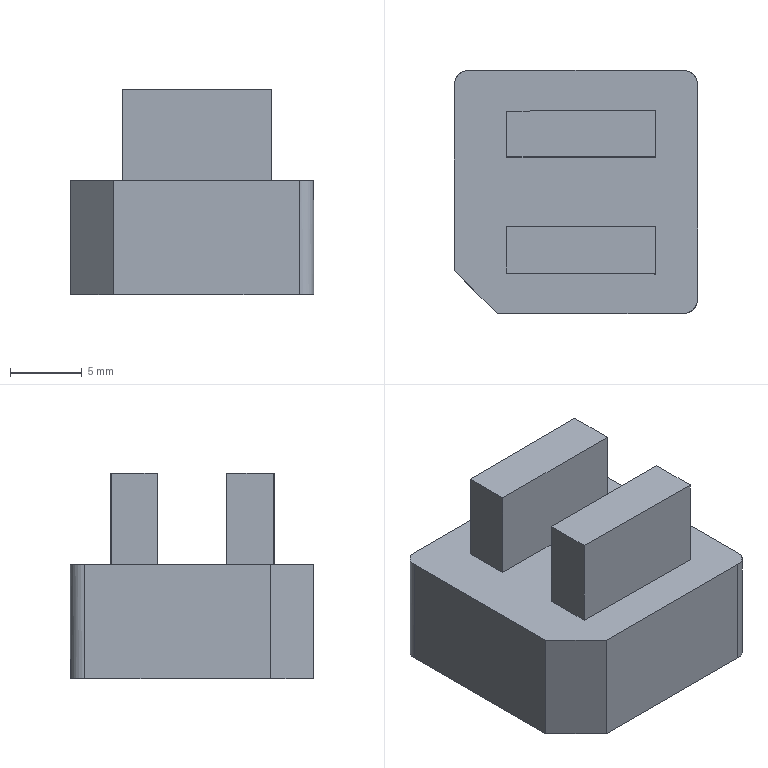NC program | PowerMill | posted with a generic post | part box 17 x 17 x 14.396 mm
Lines 6401 to 7228 of 69084:
N6498 M6
N6499 S8500 M03
N6500 G00 G90 X0.0 Y0.0
N6501 G43 Z11.796 H3
N6502
N6503 G05 P10000 R8
N6504 X16.0978 Y7.7721
N6505 Z0.9258
N6506 G01 Z-0.2742 F360.0
N6507 X10.935 Y6.6897 F600.0
N6508 X-10.201 Y6.6954
N6509 X-10.2583 Y6.3547
N6510 X-10.2871 Y6.09
N6511 X-10.2995 Y5.8905
N6512 X-10.306 Y5.6906
N6513 X-10.3062 Y2.5276
N6514 X-10.3013 Y2.218
N6515 X11.0232 Y2.2123
N6516 X11.002 Y1.899
N6517 X10.9563 Y1.5472
N6518 X10.9195 Y1.3451
N6519 G02 X10.6744 Y0.4925 I-5.5402 J1.1307
N6520 G01 X10.5807 Y0.2614
N6521 X10.4599 Y-0.0004
N6522 X10.5886 Y-0.2788
N6523 X10.7202 Y-0.6192
N6524 X10.788 Y-0.8255
N6525 G02 X11.0078 Y-1.961 I-5.3064 J-1.6164
N6526 G01 X11.0245 Y-2.2651
N6527 X-10.3525 Y-2.2594
N6528 X-10.3562 Y-2.5278
N6529 Y-5.6906
N6530 X-10.3462 Y-6.0157
N6531 X-10.3293 Y-6.2193
N6532 X-10.3062 Y-6.4224
N6533 X-10.2534 Y-6.7368
N6534 X10.9345 Y-6.7424
N6535 G00 Z11.796
N6536 G05 P0
N6537 (---------------)
N6538 ( END TOOLPATH : 精公基准台01-平坦面平行-D10 )
N6539 (---------------)
N6540 ( START TOOLPATH : 精公基准台01-基准面偏置-D10 )
N6541 (---------------)
N6542 G00 X0.0 Y0.0 Z9.7958
N6543 G05 P10000 R8
N6544 X6.0808 Y19.2543
N6545 Z-5.4
N6546 G01 Z-6.6 F360.0
N6547 Y13.9793 F600.0
N6548 X0.2833 Y11.0423
N6549 X5.6668 Y11.0687
N6550 X6.0039 Y11.0503
N6551 X6.2562 Y11.0233
N6552 X6.5169 Y10.982
N6553 X6.8002 Y10.9224
N6554 X7.0836 Y10.8461
N6555 X7.3669 Y10.7534
N6556 X7.6502 Y10.6422
N6557 X7.99 Y10.4837
N6558 X8.2169 Y10.3614
N6559 X8.5003 Y10.1874
N6560 X8.7836 Y9.9881
N6561 X8.876 Y9.917
N6562 X9.1125 Y9.7198
N6563 X9.3503 Y9.4961
N6564 X9.4909 Y9.3503
N6565 X9.718 Y9.0892
N6566 X9.9496 Y8.7836
N6567 X10.1358 Y8.5003
N6568 X10.2977 Y8.2169
N6569 X10.4837 Y7.8312
N6570 X10.5584 Y7.6502
N6571 X10.6604 Y7.3669
N6572 X10.7446 Y7.0836
N6573 X10.8124 Y6.8002
N6574 X10.8644 Y6.5169
N6575 X10.9009 Y6.2335
N6576 X10.922 Y5.9502
N6577 X10.9283 Y5.3835
N6578 X10.9259 Y2.2667
N6579 X10.9098 Y1.9834
N6580 X10.8789 Y1.7001
N6581 X10.832 Y1.4167
N6582 X10.7699 Y1.1334
N6583 X10.6912 Y0.85
N6584 X10.5964 Y0.5689
N6585 X10.5177 Y0.3729
N6586 G03 X10.5175 Y-0.3719 I0.928 J-0.3726
N6587 G01 X10.5969 Y-0.5699
N6588 X10.6915 Y-0.85
N6589 X10.7699 Y-1.1334
N6590 X10.8323 Y-1.4167
N6591 X10.8789 Y-1.7001
N6592 X10.9098 Y-1.9834
N6593 X10.9259 Y-2.2667
N6594 X10.9283 Y-5.3835
N6595 X10.9242 Y-5.9502
N6596 X10.9059 Y-6.2335
N6597 X10.8719 Y-6.5169
N6598 X10.8229 Y-6.8002
N6599 X10.7576 Y-7.0836
N6600 X10.6764 Y-7.3669
N6601 X10.5775 Y-7.6502
N6602 X10.4837 Y-7.881
N6603 X10.324 Y-8.2169
N6604 X10.1659 Y-8.5003
N6605 X9.9842 Y-8.7836
N6606 X9.917 Y-8.8793
N6607 X9.7384 Y-9.1141
N6608 X9.5365 Y-9.3503
N6609 X9.3503 Y-9.5459
N6610 X9.1436 Y-9.7417
N6611 X8.9383 Y-9.917
N6612 X8.7836 Y-10.0379
N6613 X8.5003 Y-10.2372
N6614 X8.2169 Y-10.4109
N6615 X8.0852 Y-10.4837
N6616 X7.8677 Y-10.5939
N6617 X7.6502 Y-10.692
N6618 X7.3669 Y-10.8029
N6619 X7.0836 Y-10.8959
N6620 X6.8002 Y-10.9717
N6621 X6.5169 Y-11.0315
N6622 X6.4076 Y-11.0503
N6623 X5.9502 Y-11.1046
N6624 X5.6668 Y-11.1183
N6625 X-4.8168 Y-11.0653
N6626 X-5.2709 Y-11.0503
N6627 X-5.3835 Y-11.0409
N6628 X-5.6668 Y-11.0065
N6629 X-5.9502 Y-10.9568
N6630 X-6.2335 Y-10.891
N6631 X-6.5169 Y-10.8088
N6632 X-6.8002 Y-10.7091
N6633 X-7.0836 Y-10.5913
N6634 X-7.3085 Y-10.4837
N6635 X-7.6502 Y-10.2947
N6636 X-7.9242 Y-10.1184
N6637 X-8.2169 Y-9.902
N6638 X-8.5003 Y-9.6613
N6639 X-8.6606 Y-9.509
N6640 X-8.8146 Y-9.3503
N6641 X-9.0605 Y-9.0669
N6642 X-9.2745 Y-8.7836
N6643 X-9.3503 Y-8.6729
N6644 X-9.4944 Y-8.4449
N6645 X-9.6234 Y-8.2169
N6646 X-9.764 Y-7.9336
N6647 X-9.8846 Y-7.6502
N6648 X-10.0005 Y-7.3244
N6649 X-10.0714 Y-7.0836
N6650 X-10.1394 Y-6.8002
N6651 X-10.1917 Y-6.5169
N6652 X-10.2284 Y-6.2335
N6653 X-10.2498 Y-5.9502
N6654 X-10.2565 Y-5.3835
N6655 X-10.2538 Y-2.2667
N6656 X-10.2379 Y-1.9834
N6657 X-10.2069 Y-1.7001
N6658 X-10.1602 Y-1.4167
N6659 X-10.098 Y-1.1334
N6660 X-10.0194 Y-0.85
N6661 X-9.917 Y-0.5487
N6662 X-9.8203 Y-0.3092
N6663 G03 X-9.8153 Y0.4265 I-0.9274 J0.3742
N6664 G01 X-9.917 Y0.6887
N6665 X-9.9693 Y0.85
N6666 X-10.048 Y1.1334
N6667 X-10.1101 Y1.4167
N6668 X-10.1566 Y1.7001
N6669 X-10.1879 Y1.9834
N6670 X-10.2039 Y2.2667
N6671 X-10.2064 Y5.3835
N6672 X-10.1973 Y5.9502
N6673 X-10.173 Y6.2335
N6674 X-10.1336 Y6.5169
N6675 X-10.0788 Y6.8002
N6676 X-10.0077 Y7.0836
N6677 X-9.917 Y7.3757
N6678 X-9.8149 Y7.6502
N6679 X-9.6907 Y7.9336
N6680 X-9.5465 Y8.2169
N6681 X-9.3503 Y8.547
N6682 X-9.189 Y8.7836
N6683 X-8.9985 Y9.0319
N6684 X-8.7836 Y9.2803
N6685 X-8.7177 Y9.3503
N6686 X-8.4673 Y9.5962
N6687 X-8.2169 Y9.8127
N6688 X-8.0841 Y9.917
N6689 X-7.8672 Y10.0737
N6690 X-7.6502 Y10.2147
N6691 X-7.4034 Y10.3581
N6692 X-7.0836 Y10.5191
N6693 X-6.8002 Y10.6404
N6694 X-6.5169 Y10.7429
N6695 X-6.2335 Y10.8284
N6696 X-5.9502 Y10.8968
N6697 X-5.6668 Y10.9493
N6698 X-5.3835 Y10.9864
N6699 X-5.1002 Y11.0088
N6700 X-4.8168 Y11.0155
N6701 X0.2833 Y11.0423
N6702 G00 Z9.7958
N6703 G05 P0
N6704 (---------------)
N6705 ( END TOOLPATH : 精公基准台01-基准面偏置-D10 )
N6706 (---------------)
N6707 ( START TOOLPATH : 精公基准台01-外形侧光-D10 )
N6708 (---------------)
N6709 G00 X0.0 Y0.0 Z10.796
N6710 G05 P10000 R8
N6711 X10.9971 Y-1.8364
N6712 Z-5.37
N6713 G01 Z-6.57 F360.0
N6714 G03 X10.5579 Y-2.8971 I1.0608 J-1.0606 F600.0
N6715 G01 X10.5582 Y-5.6597
N6716 G02 X8.5847 Y-9.7236 I-5.0121 J-0.0773
N6717 G02 X5.4763 Y-10.7491 I-3.0386 J3.9866
N6718 G01 X0.2734 Y-10.7218
N6719 X-4.9314 Y-10.6945
N6720 G02 X-9.8863 Y-5.6592 I0.0553 J5.0099
N6721 G01 X-9.8859 Y-2.3708
N6722 G02 X-9.2883 Y-0.0577 I4.9637 J-0.0487
N6723 G03 X-9.2858 Y0.1463 I-0.1936 J0.1043
N6724 G02 X-9.8359 Y2.3732 I4.46 J2.2832
N6725 G01 X-9.8362 Y5.6611
N6726 G02 X-4.9294 Y10.6443 I5.01 J-0.0258
N6727 G01 X5.4771 Y10.6994
N6728 G02 X10.5582 Y5.6592 I0.0702 J-5.0105
N6729 G01 X10.5578 Y2.3708
N6730 G02 X9.9849 Y0.1035 I-4.9764 J0.0514
N6731 G03 X9.9853 Y-0.1044 I0.1941 J-0.1036
N6732 G02 X10.5579 Y-2.3732 I-4.3942 J-2.3155
N6733 G01 Y-2.8971
N6734 G03 X10.9973 Y-3.9577 I1.5 J0.0001
N6735 G01 X10.9171 Y-1.7818
N6736 G03 X10.4779 Y-2.8425 I1.0608 J-1.0605
N6737 G01 X10.4782 Y-5.6592
N6738 G02 X8.5147 Y-9.6763 I-4.932 J-0.0778
N6739 G02 X5.4767 Y-10.6691 I-2.9685 J3.9393
N6740 G01 X0.2738 Y-10.6418
N6741 X-4.929 Y-10.6145
N6742 X-4.9297
N6743 X-4.9305
N6744 G02 X-9.8063 Y-5.6592 I0.0544 J4.9299
N6745 G01 X-9.8059 Y-2.3732
N6746 G02 X-9.2178 Y-0.0957 I4.8836 J-0.0463
N6747 G03 X-9.2145 Y0.1826 I-0.2641 J0.1423
N6748 G02 X-9.7559 Y2.3732 I4.3882 J2.2467
N6749 G01 X-9.7562 Y5.6592
N6750 G02 X-4.929 Y10.5643 I4.9299 J-0.0239
N6751 G01 X5.4767 Y10.6194
N6752 G02 X10.4782 Y5.6592 I0.0706 J-4.9305
N6753 G01 X10.4778 Y2.3732
N6754 G02 X9.9143 Y0.1411 I-4.8961 J0.0489
N6755 G03 X9.9149 Y-0.1424 I0.2647 J-0.1412
N6756 G02 X10.4779 Y-2.3732 I-4.3213 J-2.2769
N6757 G01 Y-2.8425
N6758 G03 X10.9173 Y-3.9031 I1.5 J0.0002
N6759 G00 Z10.796
N6760 G05 P0
N6761 (---------------)
N6762 ( END TOOLPATH : 精公基准台01-外形侧光-D10 )
N6763 (---------------)
N6764 ( START TOOLPATH : 精公基准台01-基准台侧光-D10 )
N6765 (---------------)
N6766 G00 X0.0 Y0.0 Z9.7958
N6767 G05 P10000 R8
N6768 X13.8165 Y-16.5994
N6769 Z-13.3
N6770 G01 Z-14.5 F360.0
N6771 G03 X10.9785 Y-12.4828 I-1.419 J2.0583 F600.0
N6772 G01 X10.7944 Y-12.6097
N6773 X10.7928 Y-12.6108
N6774 X10.7913 Y-12.6118
N6775 X10.6278 Y-12.7137
N6776 X10.6266 Y-12.7144
N6777 X10.6255 Y-12.715
N6778 X10.4729 Y-12.8035
N6779 X10.4714 Y-12.8043
N6780 X10.4698 Y-12.8052
N6781 X10.1537 Y-12.9703
N6782 X10.1516 Y-12.9713
N6783 X10.1495 Y-12.9723
N6784 X9.8333 Y-13.1144
N6785 X9.8312 Y-13.1153
N6786 X9.8291 Y-13.1162
N6787 X9.5129 Y-13.237
N6788 X9.5107 Y-13.2379
N6789 X9.5084 Y-13.2386
N6790 X9.1403 Y-13.3544
N6791 X9.1383 Y-13.3551
N6792 X9.1361 Y-13.3556
N6793 X8.8719 Y-13.4232
N6794 X8.8699 Y-13.4237
N6795 X8.8678 Y-13.4241
N6796 X8.5517 Y-13.4876
N6797 X8.5497 Y-13.488
N6798 X8.5478 Y-13.4883
N6799 X8.2317 Y-13.5357
N6800 X8.2294 Y-13.536
N6801 X8.2271 Y-13.5363
N6802 X7.911 Y-13.5653
N6803 X7.909 Y-13.5655
N6804 X7.9071 Y-13.5656
N6805 X7.5909 Y-13.5792
N6806 X7.5892
N6807 X7.5875
N6808 X-5.3745 Y-13.58
N6809 X-5.3749
N6810 X-5.3754
N6811 X-5.6915 Y-13.5764
N6812 X-5.6939 Y-13.5763
N6813 X-5.6962 Y-13.5762
N6814 X-6.0124 Y-13.5541
N6815 X-6.0149 Y-13.5538
N6816 X-6.0174 Y-13.5535
N6817 X-6.3336 Y-13.5111
N6818 X-6.3361 Y-13.5107
N6819 X-6.3386 Y-13.5103
N6820 X-6.6548 Y-13.447
N6821 X-6.6573 Y-13.4464
N6822 X-6.6598 Y-13.4458
N6823 X-6.976 Y-13.3608
N6824 X-6.9785 Y-13.3601
N6825 X-6.981 Y-13.3593
N6826 X-7.2972 Y-13.2514
N6827 X-7.2997 Y-13.2505
N6828 X-7.3022 Y-13.2495
N6829 X-7.6184 Y-13.1172
N6830 X-7.6203 Y-13.1163
N6831 X-7.6223 Y-13.1154
N6832 X-7.791 Y-13.034
N6833 X-7.7923 Y-13.0334
N6834 X-7.7936 Y-13.0328
N6835 X-7.9409 Y-12.9551
N6836 X-7.9428 Y-12.9541
N6837 X-7.9447 Y-12.953
N6838 X-8.2608 Y-12.7643
N6839 X-8.2624 Y-12.7633
N6840 X-8.2639 Y-12.7623
N6841 X-8.3391 Y-12.7126
N6842 X-8.3404 Y-12.7117
N6843 X-8.3417 Y-12.7108
N6844 X-8.5826 Y-12.5378
N6845 X-8.5843 Y-12.5365
N6846 X-8.5859 Y-12.5352
N6847 X-8.7646 Y-12.3921
N6848 X-8.7659 Y-12.3911
N6849 X-8.7671 Y-12.39
N6850 X-8.9046 Y-12.2703
N6851 X-8.906 Y-12.269
N6852 X-8.9074 Y-12.2678
N6853 X-9.1128 Y-12.0714
N6854 X-9.1135 Y-12.0707
N6855 X-9.1141 Y-12.0701
N6856 X-12.0701 Y-9.1141
N6857 X-12.0707 Y-9.1135
N6858 X-12.0714 Y-9.1128
N6859 X-12.2678 Y-8.9074
N6860 X-12.269 Y-8.906
N6861 X-12.2703 Y-8.9046
N6862 X-12.39 Y-8.7671
N6863 X-12.3911 Y-8.7659
N6864 X-12.3921 Y-8.7646
N6865 X-12.5352 Y-8.5859
N6866 X-12.5365 Y-8.5843
N6867 X-12.5378 Y-8.5826
N6868 X-12.7108 Y-8.3417
N6869 X-12.7117 Y-8.3404
N6870 X-12.7126 Y-8.3391
N6871 X-12.7623 Y-8.2639
N6872 X-12.7633 Y-8.2624
N6873 X-12.7643 Y-8.2608
N6874 X-12.953 Y-7.9447
N6875 X-12.9541 Y-7.9428
N6876 X-12.9551 Y-7.9409
N6877 X-13.0328 Y-7.7936
N6878 X-13.0334 Y-7.7923
N6879 X-13.034 Y-7.791
N6880 X-13.1154 Y-7.6223
N6881 X-13.1163 Y-7.6203
N6882 X-13.1172 Y-7.6184
N6883 X-13.2495 Y-7.3022
N6884 X-13.2505 Y-7.2998
N6885 X-13.2514 Y-7.2973
N6886 X-13.3538 Y-6.9989
N6887 X-13.3546 Y-6.9964
N6888 X-13.3553 Y-6.9939
N6889 X-13.4457 Y-6.66
N6890 X-13.4464 Y-6.6574
N6891 X-13.447 Y-6.6548
N6892 X-13.5103 Y-6.3386
N6893 X-13.5107 Y-6.3361
N6894 X-13.5111 Y-6.3336
N6895 X-13.5535 Y-6.0174
N6896 X-13.5538 Y-6.0149
N6897 X-13.5541 Y-6.0124
N6898 X-13.5762 Y-5.6962
N6899 X-13.5763 Y-5.6939
N6900 X-13.5764 Y-5.6915
N6901 X-13.58 Y-5.3754
N6902 Y-5.3749
N6903 Y-5.3745
N6904 X-13.5792 Y7.5875
N6905 Y7.5891
N6906 Y7.5907
N6907 X-13.5663 Y7.9069
N6908 X-13.5662 Y7.909
N6909 X-13.5661 Y7.9111
N6910 X-13.5363 Y8.2273
N6911 X-13.536 Y8.2294
N6912 X-13.5357 Y8.2315
N6913 X-13.489 Y8.5476
N6914 X-13.4887 Y8.5498
N6915 X-13.4883 Y8.5519
N6916 X-13.424 Y8.868
N6917 X-13.4236 Y8.87
N6918 X-13.4232 Y8.8719
N6919 X-13.3556 Y9.1361
N6920 X-13.3551 Y9.1383
N6921 X-13.3544 Y9.1404
N6922 X-13.2385 Y9.5084
N6923 X-13.2377 Y9.5107
N6924 X-13.2369 Y9.5129
N6925 X-13.1162 Y9.8291
N6926 X-13.1155 Y9.8308
N6927 X-13.1148 Y9.8324
N6928 X-13.0353 Y10.0152
N6929 X-13.0349 Y10.0162
N6930 X-13.0344 Y10.0173
N6931 X-12.9716 Y10.1507
N6932 X-12.9708 Y10.1522
N6933 X-12.9701 Y10.1537
N6934 X-12.8052 Y10.4698
N6935 X-12.8044 Y10.4714
N6936 X-12.8035 Y10.4729
N6937 X-12.715 Y10.6255
N6938 X-12.7144 Y10.6266
N6939 X-12.7137 Y10.6277
N6940 X-12.612 Y10.7912
N6941 X-12.611 Y10.7928
N6942 X-12.6099 Y10.7943
N6943 X-12.3956 Y11.1054
N6944 X-12.394 Y11.1076
N6945 X-12.3924 Y11.1097
N6946 X-12.1383 Y11.4309
N6947 X-12.1372 Y11.4322
N6948 X-12.1362 Y11.4335
N6949 X-12.0741 Y11.5055
N6950 X-12.0732 Y11.5065
N6951 X-12.0722 Y11.5076
N6952 X-11.846 Y11.7518
N6953 X-11.845 Y11.7529
N6954 X-11.8439 Y11.754
N6955 X-11.754 Y11.8439
N6956 X-11.7529 Y11.845
N6957 X-11.7517 Y11.846
N6958 X-11.5074 Y12.0722
N6959 X-11.5062 Y12.0733
N6960 X-11.505 Y12.0744
N6961 X-11.4332 Y12.1357
N6962 X-11.4321 Y12.1367
N6963 X-11.431 Y12.1376
N6964 X-11.1148 Y12.3886
N6965 X-11.1127 Y12.3902
N6966 X-11.1105 Y12.3918
N6967 X-10.7944 Y12.6097
N6968 X-10.7928 Y12.6108
N6969 X-10.7913 Y12.6118
N6970 X-10.6278 Y12.7137
N6971 X-10.6266 Y12.7144
N6972 X-10.6255 Y12.715
N6973 X-10.4729 Y12.8035
N6974 X-10.4714 Y12.8043
N6975 X-10.4698 Y12.8052
N6976 X-10.1537 Y12.9703
N6977 X-10.1516 Y12.9713
N6978 X-10.1495 Y12.9723
N6979 X-9.8333 Y13.1144
N6980 X-9.8312 Y13.1153
N6981 X-9.8291 Y13.1162
N6982 X-9.5129 Y13.237
N6983 X-9.5108 Y13.2378
N6984 X-9.5087 Y13.2385
N6985 X-9.1926 Y13.3396
N6986 X-9.1905 Y13.3402
N6987 X-9.1884 Y13.3408
N6988 X-8.8722 Y13.4231
N6989 X-8.87 Y13.4236
N6990 X-8.8678 Y13.4241
N6991 X-8.5517 Y13.4876
N6992 X-8.5497 Y13.488
N6993 X-8.5478 Y13.4883
N6994 X-8.2317 Y13.5357
N6995 X-8.2294 Y13.536
N6996 X-8.2271 Y13.5363
N6997 X-7.911 Y13.5653
N6998 X-7.909 Y13.5655
N6999 X-7.9071 Y13.5656
N7000 X-7.5909 Y13.5792
N7001 X-7.5892
N7002 X-7.5875
N7003 X0.0
N7004 X7.5875
N7005 X7.5891
N7006 X7.5907
N7007 X7.9069 Y13.5663
N7008 X7.909 Y13.5662
N7009 X7.9111 Y13.5661
N7010 X8.2273 Y13.5363
N7011 X8.2294 Y13.536
N7012 X8.2315 Y13.5357
N7013 X8.5476 Y13.489
N7014 X8.5498 Y13.4887
N7015 X8.5519 Y13.4883
N7016 X8.868 Y13.424
N7017 X8.87 Y13.4236
N7018 X8.8719 Y13.4232
N7019 X9.1361 Y13.3556
N7020 X9.1383 Y13.3551
N7021 X9.1404 Y13.3544
N7022 X9.5084 Y13.2385
N7023 X9.5107 Y13.2377
N7024 X9.5129 Y13.2369
N7025 X9.8291 Y13.1162
N7026 X9.8308 Y13.1155
N7027 X9.8324 Y13.1148
N7028 X10.0152 Y13.0353
N7029 X10.0162 Y13.0349
N7030 X10.0173 Y13.0344
N7031 X10.1507 Y12.9716
N7032 X10.1522 Y12.9708
N7033 X10.1537 Y12.9701
N7034 X10.4698 Y12.8052
N7035 X10.4714 Y12.8044
N7036 X10.4729 Y12.8035
N7037 X10.6255 Y12.715
N7038 X10.6266 Y12.7144
N7039 X10.6277 Y12.7137
N7040 X10.7912 Y12.612
N7041 X10.7928 Y12.611
N7042 X10.7943 Y12.6099
N7043 X11.1054 Y12.3956
N7044 X11.1076 Y12.394
N7045 X11.1097 Y12.3924
N7046 X11.4309 Y12.1383
N7047 X11.4322 Y12.1372
N7048 X11.4335 Y12.1362
N7049 X11.5055 Y12.0741
N7050 X11.5065 Y12.0732
N7051 X11.5076 Y12.0722
N7052 X11.7518 Y11.846
N7053 X11.7529 Y11.845
N7054 X11.754 Y11.8439
N7055 X11.8439 Y11.754
N7056 X11.845 Y11.7529
N7057 X11.846 Y11.7517
N7058 X12.0722 Y11.5074
N7059 X12.0733 Y11.5062
N7060 X12.0744 Y11.505
N7061 X12.1357 Y11.4332
N7062 X12.1367 Y11.4321
N7063 X12.1376 Y11.431
N7064 X12.3886 Y11.1148
N7065 X12.3902 Y11.1127
N7066 X12.3918 Y11.1105
N7067 X12.6097 Y10.7944
N7068 X12.6108 Y10.7928
N7069 X12.6118 Y10.7913
N7070 X12.7137 Y10.6278
N7071 X12.7144 Y10.6266
N7072 X12.715 Y10.6255
N7073 X12.8035 Y10.4729
N7074 X12.8043 Y10.4714
N7075 X12.8052 Y10.4698
N7076 X12.9703 Y10.1537
N7077 X12.9713 Y10.1516
N7078 X12.9723 Y10.1495
N7079 X13.1144 Y9.8333
N7080 X13.1153 Y9.8312
N7081 X13.1162 Y9.8291
N7082 X13.237 Y9.5129
N7083 X13.2378 Y9.5108
N7084 X13.2385 Y9.5087
N7085 X13.3396 Y9.1926
N7086 X13.3402 Y9.1905
N7087 X13.3408 Y9.1884
N7088 X13.4231 Y8.8722
N7089 X13.4236 Y8.87
N7090 X13.4241 Y8.8678
N7091 X13.4876 Y8.5517
N7092 X13.488 Y8.5497
N7093 X13.4883 Y8.5478
N7094 X13.5357 Y8.2317
N7095 X13.536 Y8.2294
N7096 X13.5363 Y8.2271
N7097 X13.5653 Y7.911
N7098 X13.5655 Y7.909
N7099 X13.5656 Y7.9071
N7100 X13.5792 Y7.5909
N7101 Y7.5892
N7102 Y7.5875
N7103 Y-7.5875
N7104 Y-7.5891
N7105 Y-7.5907
N7106 X13.5663 Y-7.9069
N7107 X13.5662 Y-7.909
N7108 X13.5661 Y-7.9111
N7109 X13.5363 Y-8.2273
N7110 X13.536 Y-8.2294
N7111 X13.5357 Y-8.2315
N7112 X13.489 Y-8.5476
N7113 X13.4887 Y-8.5498
N7114 X13.4883 Y-8.5519
N7115 X13.424 Y-8.868
N7116 X13.4236 Y-8.87
N7117 X13.4232 Y-8.8719
N7118 X13.3556 Y-9.1361
N7119 X13.3551 Y-9.1383
N7120 X13.3544 Y-9.1404
N7121 X13.2385 Y-9.5084
N7122 X13.2377 Y-9.5107
N7123 X13.2369 Y-9.5129
N7124 X13.1162 Y-9.8291
N7125 X13.1155 Y-9.8308
N7126 X13.1148 Y-9.8324
N7127 X13.0353 Y-10.0152
N7128 X13.0349 Y-10.0162
N7129 X13.0344 Y-10.0173
N7130 X12.9716 Y-10.1507
N7131 X12.9708 Y-10.1522
N7132 X12.9701 Y-10.1537
N7133 X12.8052 Y-10.4698
N7134 X12.8044 Y-10.4714
N7135 X12.8035 Y-10.4729
N7136 X12.715 Y-10.6255
N7137 X12.7144 Y-10.6266
N7138 X12.7137 Y-10.6277
N7139 X12.612 Y-10.7912
N7140 X12.611 Y-10.7928
N7141 X12.6099 Y-10.7943
N7142 X12.3956 Y-11.1054
N7143 X12.394 Y-11.1076
N7144 X12.3924 Y-11.1097
N7145 X12.1383 Y-11.4309
N7146 X12.1372 Y-11.4322
N7147 X12.1362 Y-11.4335
N7148 X12.0741 Y-11.5055
N7149 X12.0732 Y-11.5065
N7150 X12.0722 Y-11.5076
N7151 X11.846 Y-11.7518
N7152 X11.845 Y-11.7529
N7153 X11.8439 Y-11.754
N7154 X11.754 Y-11.8439
N7155 X11.7529 Y-11.845
N7156 X11.7517 Y-11.846
N7157 X11.5074 Y-12.0722
N7158 X11.5062 Y-12.0733
N7159 X11.505 Y-12.0744
N7160 X11.4332 Y-12.1357
N7161 X11.4321 Y-12.1367
N7162 X11.431 Y-12.1376
N7163 X11.1148 Y-12.3886
N7164 X11.1127 Y-12.3902
N7165 X11.1105 Y-12.3918
N7166 X10.9785 Y-12.4828
N7167 G03 X13.8165 Y-16.5993 I1.419 J-2.0583
N7168 G01 X13.765 Y-16.5377
N7169 G03 X10.9271 Y-12.4211 I-1.419 J2.0583
N7170 G01 X10.749 Y-12.5439
N7171 X10.5854 Y-12.6458
N7172 X10.4328 Y-12.7343
N7173 X10.1167 Y-12.8994
N7174 X9.8005 Y-13.0415
N7175 X9.4844 Y-13.1623
N7176 X9.1163 Y-13.2781
N7177 X8.8521 Y-13.3457
N7178 X8.5359 Y-13.4092
N7179 X8.2198 Y-13.4566
N7180 X7.9036 Y-13.4857
N7181 X7.5875 Y-13.4992
N7182 X7.2714 Y-13.5
N7183 X-5.3745
N7184 X-5.6906 Y-13.4964
N7185 X-6.0068 Y-13.4743
N7186 X-6.3229 Y-13.4318
N7187 X-6.6391 Y-13.3685
N7188 X-6.9552 Y-13.2836
N7189 X-7.2714 Y-13.1757
N7190 X-7.5875 Y-13.0434
N7191 X-7.7563 Y-12.962
N7192 X-7.9036 Y-12.8844
N7193 X-8.2198 Y-12.6956
N7194 X-8.295 Y-12.6458
N7195 X-8.5359 Y-12.4728
N7196 X-8.7146 Y-12.3297
N7197 X-8.8521 Y-12.2099
N7198 X-9.0575 Y-12.0135
N7199 X-12.0135 Y-9.0575
N7200 X-12.2099 Y-8.8521
N7201 X-12.3297 Y-8.7146
N7202 X-12.4728 Y-8.5359
N7203 X-12.6458 Y-8.295
N7204 X-12.6956 Y-8.2198
N7205 X-12.8844 Y-7.9036
N7206 X-12.962 Y-7.7563
N7207 X-13.0434 Y-7.5875
N7208 X-13.1757 Y-7.2714
N7209 X-13.2781 Y-6.973
N7210 X-13.3685 Y-6.6391
N7211 X-13.4318 Y-6.3229
N7212 X-13.4743 Y-6.0068
N7213 X-13.4964 Y-5.6906
N7214 X-13.5 Y-5.3745
N7215 Y7.2714
N7216 X-13.4992 Y7.5875
N7217 X-13.4864 Y7.9036
N7218 X-13.4566 Y8.2198
N7219 X-13.4099 Y8.5359
N7220 X-13.3456 Y8.8521
N7221 X-13.2781 Y9.1163
N7222 X-13.1622 Y9.4844
N7223 X-13.0415 Y9.8005
N7224 X-12.962 Y9.9832
N7225 X-12.8992 Y10.1167
N7226 X-12.7343 Y10.4328
N7227 X-12.6458 Y10.5854
N7228 X-12.544 Y10.749
N7229 X-12.3297 Y11.06
N7230 X-12.0756 Y11.3812
N7231 X-12.0135 Y11.4532
N7232 X-11.7873 Y11.6974
N7233 X-11.6974 Y11.7873
N7234 X-11.4531 Y12.0135
N7235 X-11.3812 Y12.0749
N7236 X-11.0651 Y12.3259
N7237 X-10.749 Y12.5439
N7238 X-10.5854 Y12.6458
N7239 X-10.4328 Y12.7343
N7240 X-10.1167 Y12.8994
N7241 X-9.8005 Y13.0415
N7242 X-9.4844 Y13.1623
N7243 X-9.1682 Y13.2634
N7244 X-8.8521 Y13.3457
N7245 X-8.5359 Y13.4092
N7246 X-8.2198 Y13.4566
N7247 X-7.9036 Y13.4857
N7248 X-7.5875 Y13.4992
N7249 X-7.2714 Y13.5
N7250 X0.0
N7251 X7.2714
N7252 X7.5875 Y13.4992
N7253 X7.9036 Y13.4864
N7254 X8.2198 Y13.4566
N7255 X8.5359 Y13.4099
N7256 X8.8521 Y13.3456
N7257 X9.1163 Y13.2781
N7258 X9.4844 Y13.1622
N7259 X9.8005 Y13.0415
N7260 X9.9832 Y12.962
N7261 X10.1167 Y12.8992
N7262 X10.4328 Y12.7343
N7263 X10.5854 Y12.6458
N7264 X10.749 Y12.544
N7265 X11.06 Y12.3297
N7266 X11.3812 Y12.0756
N7267 X11.4532 Y12.0135
N7268 X11.6974 Y11.7873
N7269 X11.7873 Y11.6974
N7270 X12.0135 Y11.4531
N7271 X12.0749 Y11.3812
N7272 X12.3259 Y11.0651
N7273 X12.5439 Y10.749
N7274 X12.6458 Y10.5854
N7275 X12.7343 Y10.4328
N7276 X12.8994 Y10.1167
N7277 X13.0415 Y9.8005
N7278 X13.1623 Y9.4844
N7279 X13.2634 Y9.1682
N7280 X13.3457 Y8.8521
N7281 X13.4092 Y8.5359
N7282 X13.4566 Y8.2198
N7283 X13.4857 Y7.9036
N7284 X13.4992 Y7.5875
N7285 X13.5 Y7.2714
N7286 Y-7.2714
N7287 X13.4992 Y-7.5875
N7288 X13.4864 Y-7.9036
N7289 X13.4566 Y-8.2198
N7290 X13.4099 Y-8.5359
N7291 X13.3456 Y-8.8521
N7292 X13.2781 Y-9.1163
N7293 X13.1622 Y-9.4844
N7294 X13.0415 Y-9.8005
N7295 X12.962 Y-9.9832
N7296 X12.8992 Y-10.1167
N7297 X12.7343 Y-10.4328
N7298 X12.6458 Y-10.5854
N7299 X12.544 Y-10.749
N7300 X12.3297 Y-11.06
N7301 X12.0756 Y-11.3812
N7302 X12.0135 Y-11.4532
N7303 X11.7873 Y-11.6974
N7304 X11.6974 Y-11.7873
N7305 X11.4531 Y-12.0135
N7306 X11.3812 Y-12.0749
N7307 X11.0651 Y-12.3259
N7308 X10.9271 Y-12.4211
N7309 G03 X13.765 Y-16.5377 I1.4189 J-2.0583
N7310 G00 Z9.7958
N7311 G05 P0
N7312 (---------------)
N7313 ( END TOOLPATH : 精公基准台01-基准台侧光-D10 )
N7314 (---------------)
N7315
N7316 M05
N7317 G53 Z0.0
N7318 (---------------)
N7319 ( START TOOLPATH : 精公精光01-等高-D3 )
N7320 (---------------)
N7321 ( TOOL NO.    :10 )
N7322 ( TOOL TYPE   : ENDMILL)
N7323 ( TOOL ID     : D3_1_1)
N7324 ( TOOL DIA    : 3.0 LENGTH 61.56)
N7325 T10